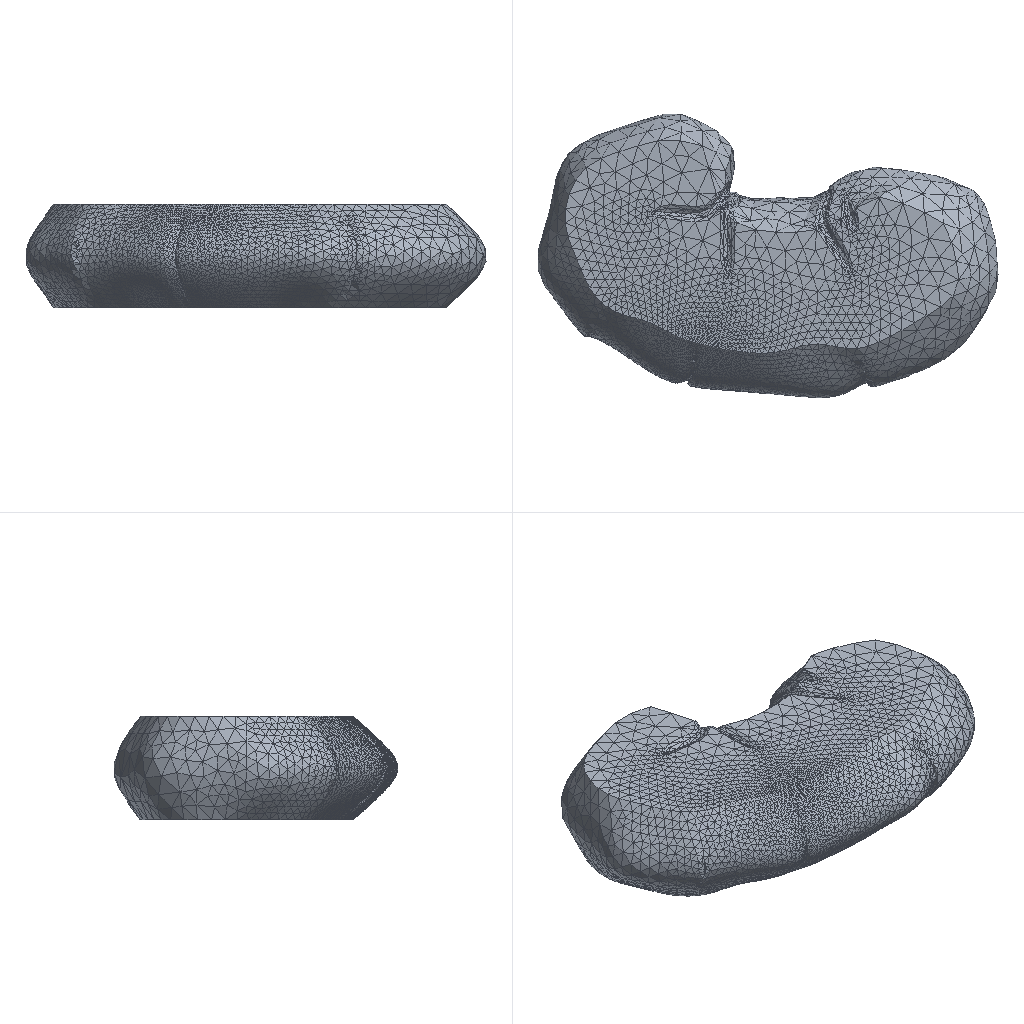Simulation study | abaqus
Set-up summary:
category,name,step,type,value,unit,region
solver,abaqus
solver,version,,,Abaqus/Explicit 2020
units,not stated in the deck,,not stated
analysis,deck,,transient,transient
load_step,Step-1,Step-1,transient,nlgeom=True
contact,interactions,,,general=1 pairs=1 ties=0
load_step,requested,,,1
mesh,nodes,,,15622
mesh,elements,,,77471
element_type,C3D4,,solid,76591
element_type,R3D4,,rigid,880
load,load commands in deck,,count,2
bc,support commands in deck,,count,7
material,MATERIAL-1,,in results
check,setup vs results,,match,"per instance, exact: element labels, types and connectivity; labels of the nodes the elements use; coordinates of those nodes at SINGLE_PRECISION in 2 of 2 instance(s)"
Results summary:
result,step,Step-1,completed,increments=38190 time=0.1/0.1
result,analysis,,,transient
result,last_loadstep,,,1
result,analysis steps,,count,1
result,primary field,,,U
result,reaction total,,FX,-31.49,model units
result,reaction total,,FY,1.598,model units
result,reaction total,,FZ,8.92,model units